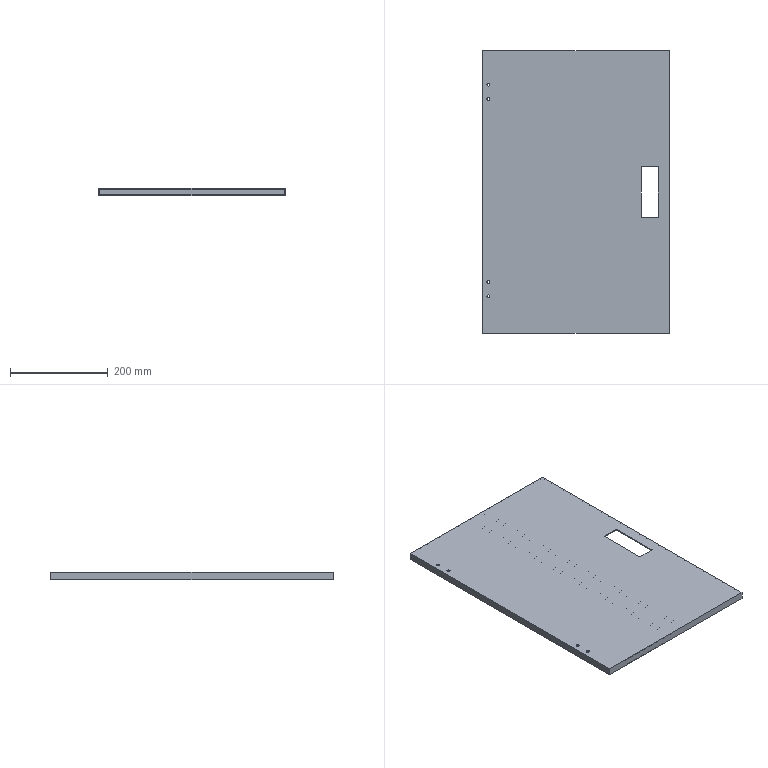Part | STEP file | Bottom door | 2 solids | 46 faces | box 382.5 x 579 x 15 mm | volume 596109 mm3 | plane 38 | cylinder 8 | commonest cylinder face diameters 6.2 x8